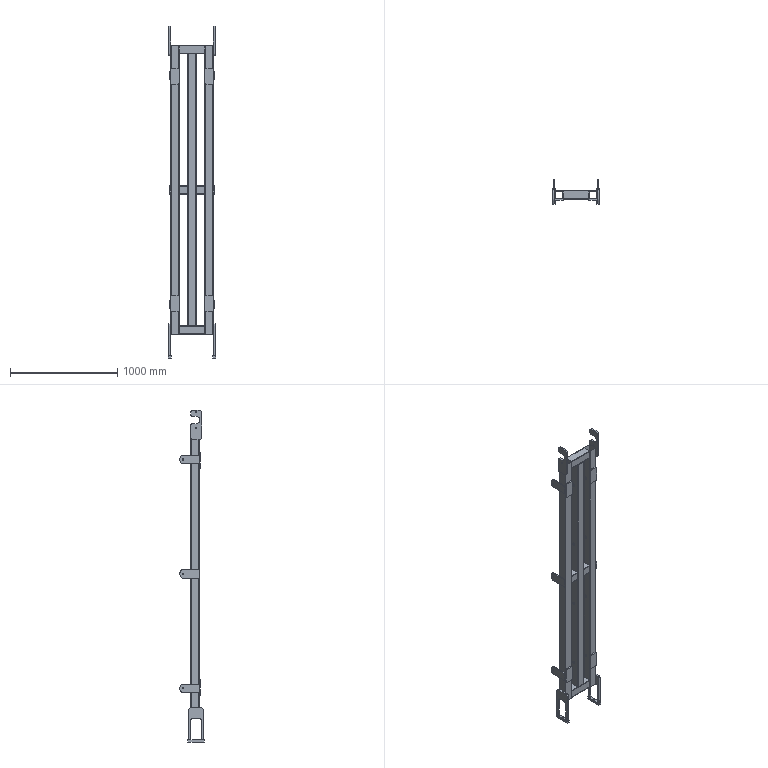Part | STEP file | 23 solids | 414 faces | box 442 x 225 x 3100 mm | volume 10604671 mm3 | cylinder 198 | plane 184 | cone 32 | commonest cylinder face diameters 26 x40 4 x28 10 x28 20 x16 50 x16 11 x12